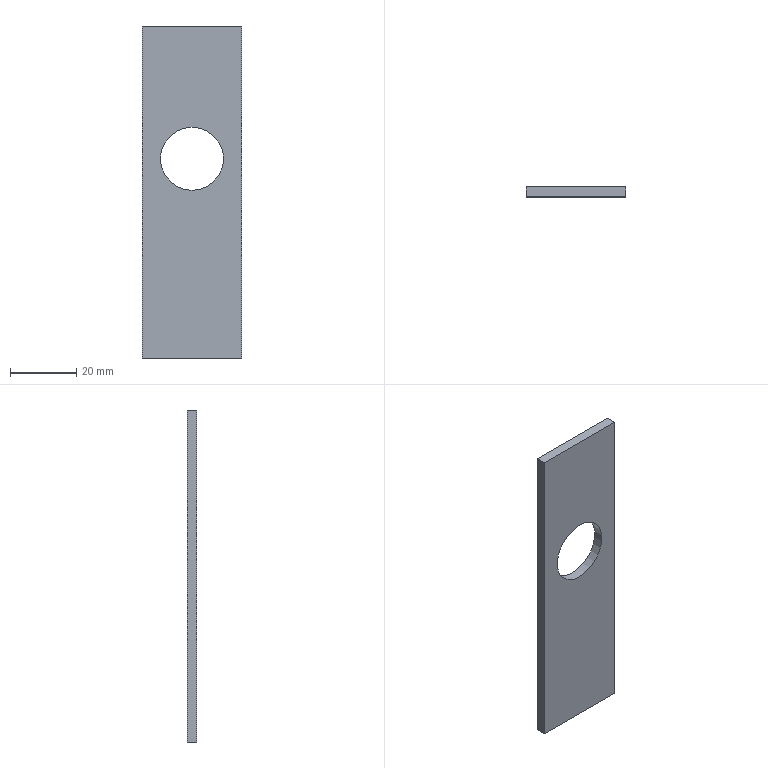Part | STEP file | 7471205 | 1 solid | 7 faces | box 30 x 3 x 100 mm | volume 8149 mm3 | plane 6 | cylinder 1 | commonest cylinder face diameters 19 x1
STEP:
#1=CARTESIAN_POINT('',(0.,0.,0.));
#2=DIRECTION('',(0.,0.,1.));
#3=DIRECTION('',(1.,0.,0.));
#4=AXIS2_PLACEMENT_3D('',#1,#2,#3);
#5=CARTESIAN_POINT('',(-15.,0.,-50.));
#6=VERTEX_POINT('',#5);
#7=CARTESIAN_POINT('',(-15.,0.,50.));
#8=VERTEX_POINT('',#7);
#9=CARTESIAN_POINT('',(-15.,0.,-50.));
#10=DIRECTION('',(0.,0.,1.));
#11=VECTOR('',#10,1.);
#12=LINE('',#9,#11);
#13=CARTESIAN_POINT('',(-15.,3.,-50.));
#14=DIRECTION('',(1.,0.,0.));
#15=DIRECTION('',(0.,0.,-1.));
#16=AXIS2_PLACEMENT_3D('',#13,#14,#15);
#17=PLANE('',#16);
#18=CARTESIAN_POINT('',(0.,-3.));
#19=DIRECTION('',(-1.,0.));
#20=VECTOR('',#19,1.);
#21=LINE('',#18,#20);
#22=(GEOMETRIC_REPRESENTATION_CONTEXT(2)PARAMETRIC_REPRESENTATION_CONTEXT()REPRESENTATION_CONTEXT('',''));
#23=DEFINITIONAL_REPRESENTATION('',(#21),#22);
#24=PCURVE('',#17,#23);
#25=CARTESIAN_POINT('',(0.,0.,0.));
#26=DIRECTION('',(0.,1.,0.));
#27=DIRECTION('',(0.,0.,1.));
#28=AXIS2_PLACEMENT_3D('',#25,#26,#27);
#29=PLANE('',#28);
#30=CARTESIAN_POINT('',(-50.,-15.));
#31=DIRECTION('',(1.,0.));
#32=VECTOR('',#31,1.);
#33=LINE('',#30,#32);
#34=(GEOMETRIC_REPRESENTATION_CONTEXT(2)PARAMETRIC_REPRESENTATION_CONTEXT()REPRESENTATION_CONTEXT('',''));
#35=DEFINITIONAL_REPRESENTATION('',(#33),#34);
#36=PCURVE('',#29,#35);
#37=SURFACE_CURVE('',#12,(#24,#36),.PCURVE_S1.);
#38=EDGE_CURVE('',#6,#8,#37,.T.);
#39=ORIENTED_EDGE('',*,*,#38,.T.);
#40=CARTESIAN_POINT('',(-15.,3.,50.));
#41=VERTEX_POINT('',#40);
#42=CARTESIAN_POINT('',(-15.,3.,50.));
#43=DIRECTION('',(0.,-1.,0.));
#44=VECTOR('',#43,1.);
#45=LINE('',#42,#44);
#46=CARTESIAN_POINT('',(-100.,0.));
#47=DIRECTION('',(0.,-1.));
#48=VECTOR('',#47,1.);
#49=LINE('',#46,#48);
#50=(GEOMETRIC_REPRESENTATION_CONTEXT(2)PARAMETRIC_REPRESENTATION_CONTEXT()REPRESENTATION_CONTEXT('',''));
#51=DEFINITIONAL_REPRESENTATION('',(#49),#50);
#52=PCURVE('',#17,#51);
#53=CARTESIAN_POINT('',(-15.,3.,50.));
#54=DIRECTION('',(0.,0.,-1.));
#55=DIRECTION('',(-1.,0.,0.));
#56=AXIS2_PLACEMENT_3D('',#53,#54,#55);
#57=PLANE('',#56);
#58=CARTESIAN_POINT('',(0.,0.));
#59=DIRECTION('',(0.,-1.));
#60=VECTOR('',#59,1.);
#61=LINE('',#58,#60);
#62=(GEOMETRIC_REPRESENTATION_CONTEXT(2)PARAMETRIC_REPRESENTATION_CONTEXT()REPRESENTATION_CONTEXT('',''));
#63=DEFINITIONAL_REPRESENTATION('',(#61),#62);
#64=PCURVE('',#57,#63);
#65=SURFACE_CURVE('',#45,(#52,#64),.PCURVE_S1.);
#66=EDGE_CURVE('',#41,#8,#65,.T.);
#67=ORIENTED_EDGE('',*,*,#66,.F.);
#68=CARTESIAN_POINT('',(-15.,3.,-50.));
#69=VERTEX_POINT('',#68);
#70=CARTESIAN_POINT('',(-15.,3.,-50.));
#71=DIRECTION('',(0.,0.,1.));
#72=VECTOR('',#71,1.);
#73=LINE('',#70,#72);
#74=CARTESIAN_POINT('',(0.,0.));
#75=DIRECTION('',(-1.,0.));
#76=VECTOR('',#75,1.);
#77=LINE('',#74,#76);
#78=(GEOMETRIC_REPRESENTATION_CONTEXT(2)PARAMETRIC_REPRESENTATION_CONTEXT()REPRESENTATION_CONTEXT('',''));
#79=DEFINITIONAL_REPRESENTATION('',(#77),#78);
#80=PCURVE('',#17,#79);
#81=CARTESIAN_POINT('',(0.,3.,0.));
#82=DIRECTION('',(0.,1.,0.));
#83=DIRECTION('',(0.,0.,1.));
#84=AXIS2_PLACEMENT_3D('',#81,#82,#83);
#85=PLANE('',#84);
#86=CARTESIAN_POINT('',(-50.,-15.));
#87=DIRECTION('',(1.,0.));
#88=VECTOR('',#87,1.);
#89=LINE('',#86,#88);
#90=(GEOMETRIC_REPRESENTATION_CONTEXT(2)PARAMETRIC_REPRESENTATION_CONTEXT()REPRESENTATION_CONTEXT('',''));
#91=DEFINITIONAL_REPRESENTATION('',(#89),#90);
#92=PCURVE('',#85,#91);
#93=SURFACE_CURVE('',#73,(#80,#92),.PCURVE_S1.);
#94=EDGE_CURVE('',#69,#41,#93,.T.);
#95=ORIENTED_EDGE('',*,*,#94,.F.);
#96=CARTESIAN_POINT('',(-15.,3.,-50.));
#97=DIRECTION('',(0.,-1.,0.));
#98=VECTOR('',#97,1.);
#99=LINE('',#96,#98);
#100=CARTESIAN_POINT('',(0.,0.));
#101=DIRECTION('',(0.,-1.));
#102=VECTOR('',#101,1.);
#103=LINE('',#100,#102);
#104=(GEOMETRIC_REPRESENTATION_CONTEXT(2)PARAMETRIC_REPRESENTATION_CONTEXT()REPRESENTATION_CONTEXT('',''));
#105=DEFINITIONAL_REPRESENTATION('',(#103),#104);
#106=PCURVE('',#17,#105);
#107=CARTESIAN_POINT('',(-15.,3.,-50.));
#108=DIRECTION('',(0.,0.,1.));
#109=DIRECTION('',(1.,0.,0.));
#110=AXIS2_PLACEMENT_3D('',#107,#108,#109);
#111=PLANE('',#110);
#112=CARTESIAN_POINT('',(0.,0.));
#113=DIRECTION('',(0.,-1.));
#114=VECTOR('',#113,1.);
#115=LINE('',#112,#114);
#116=(GEOMETRIC_REPRESENTATION_CONTEXT(2)PARAMETRIC_REPRESENTATION_CONTEXT()REPRESENTATION_CONTEXT('',''));
#117=DEFINITIONAL_REPRESENTATION('',(#115),#116);
#118=PCURVE('',#111,#117);
#119=SURFACE_CURVE('',#99,(#106,#118),.PCURVE_S1.);
#120=EDGE_CURVE('',#69,#6,#119,.T.);
#121=ORIENTED_EDGE('',*,*,#120,.T.);
#122=EDGE_LOOP('',(#39,#67,#95,#121));
#123=FACE_BOUND('',#122,.T.);
#124=ADVANCED_FACE('',(#123),#17,.F.);
#125=CARTESIAN_POINT('',(15.,0.,50.));
#126=VERTEX_POINT('',#125);
#127=CARTESIAN_POINT('',(-15.,0.,50.));
#128=DIRECTION('',(1.,0.,0.));
#129=VECTOR('',#128,1.);
#130=LINE('',#127,#129);
#131=CARTESIAN_POINT('',(0.,-3.));
#132=DIRECTION('',(-1.,0.));
#133=VECTOR('',#132,1.);
#134=LINE('',#131,#133);
#135=(GEOMETRIC_REPRESENTATION_CONTEXT(2)PARAMETRIC_REPRESENTATION_CONTEXT()REPRESENTATION_CONTEXT('',''));
#136=DEFINITIONAL_REPRESENTATION('',(#134),#135);
#137=PCURVE('',#57,#136);
#138=CARTESIAN_POINT('',(50.,-15.));
#139=DIRECTION('',(0.,1.));
#140=VECTOR('',#139,1.);
#141=LINE('',#138,#140);
#142=(GEOMETRIC_REPRESENTATION_CONTEXT(2)PARAMETRIC_REPRESENTATION_CONTEXT()REPRESENTATION_CONTEXT('',''));
#143=DEFINITIONAL_REPRESENTATION('',(#141),#142);
#144=PCURVE('',#29,#143);
#145=SURFACE_CURVE('',#130,(#137,#144),.PCURVE_S1.);
#146=EDGE_CURVE('',#8,#126,#145,.T.);
#147=ORIENTED_EDGE('',*,*,#146,.T.);
#148=CARTESIAN_POINT('',(15.,3.,50.));
#149=VERTEX_POINT('',#148);
#150=CARTESIAN_POINT('',(15.,3.,50.));
#151=DIRECTION('',(0.,-1.,0.));
#152=VECTOR('',#151,1.);
#153=LINE('',#150,#152);
#154=CARTESIAN_POINT('',(-30.,0.));
#155=DIRECTION('',(0.,-1.));
#156=VECTOR('',#155,1.);
#157=LINE('',#154,#156);
#158=(GEOMETRIC_REPRESENTATION_CONTEXT(2)PARAMETRIC_REPRESENTATION_CONTEXT()REPRESENTATION_CONTEXT('',''));
#159=DEFINITIONAL_REPRESENTATION('',(#157),#158);
#160=PCURVE('',#57,#159);
#161=CARTESIAN_POINT('',(15.,3.,-50.));
#162=DIRECTION('',(-1.,0.,0.));
#163=DIRECTION('',(0.,0.,1.));
#164=AXIS2_PLACEMENT_3D('',#161,#162,#163);
#165=PLANE('',#164);
#166=CARTESIAN_POINT('',(100.,0.));
#167=DIRECTION('',(0.,-1.));
#168=VECTOR('',#167,1.);
#169=LINE('',#166,#168);
#170=(GEOMETRIC_REPRESENTATION_CONTEXT(2)PARAMETRIC_REPRESENTATION_CONTEXT()REPRESENTATION_CONTEXT('',''));
#171=DEFINITIONAL_REPRESENTATION('',(#169),#170);
#172=PCURVE('',#165,#171);
#173=SURFACE_CURVE('',#153,(#160,#172),.PCURVE_S1.);
#174=EDGE_CURVE('',#149,#126,#173,.T.);
#175=ORIENTED_EDGE('',*,*,#174,.F.);
#176=CARTESIAN_POINT('',(-15.,3.,50.));
#177=DIRECTION('',(1.,0.,0.));
#178=VECTOR('',#177,1.);
#179=LINE('',#176,#178);
#180=CARTESIAN_POINT('',(0.,0.));
#181=DIRECTION('',(-1.,0.));
#182=VECTOR('',#181,1.);
#183=LINE('',#180,#182);
#184=(GEOMETRIC_REPRESENTATION_CONTEXT(2)PARAMETRIC_REPRESENTATION_CONTEXT()REPRESENTATION_CONTEXT('',''));
#185=DEFINITIONAL_REPRESENTATION('',(#183),#184);
#186=PCURVE('',#57,#185);
#187=CARTESIAN_POINT('',(50.,-15.));
#188=DIRECTION('',(0.,1.));
#189=VECTOR('',#188,1.);
#190=LINE('',#187,#189);
#191=(GEOMETRIC_REPRESENTATION_CONTEXT(2)PARAMETRIC_REPRESENTATION_CONTEXT()REPRESENTATION_CONTEXT('',''));
#192=DEFINITIONAL_REPRESENTATION('',(#190),#191);
#193=PCURVE('',#85,#192);
#194=SURFACE_CURVE('',#179,(#186,#193),.PCURVE_S1.);
#195=EDGE_CURVE('',#41,#149,#194,.T.);
#196=ORIENTED_EDGE('',*,*,#195,.F.);
#197=ORIENTED_EDGE('',*,*,#66,.T.);
#198=EDGE_LOOP('',(#147,#175,#196,#197));
#199=FACE_BOUND('',#198,.T.);
#200=ADVANCED_FACE('',(#199),#57,.F.);
#201=CARTESIAN_POINT('',(15.,0.,-50.));
#202=VERTEX_POINT('',#201);
#203=CARTESIAN_POINT('',(15.,0.,-50.));
#204=DIRECTION('',(0.,0.,-1.));
#205=VECTOR('',#204,1.);
#206=LINE('',#203,#205);
#207=CARTESIAN_POINT('',(0.,-3.));
#208=DIRECTION('',(-1.,0.));
#209=VECTOR('',#208,1.);
#210=LINE('',#207,#209);
#211=(GEOMETRIC_REPRESENTATION_CONTEXT(2)PARAMETRIC_REPRESENTATION_CONTEXT()REPRESENTATION_CONTEXT('',''));
#212=DEFINITIONAL_REPRESENTATION('',(#210),#211);
#213=PCURVE('',#165,#212);
#214=CARTESIAN_POINT('',(-50.,15.));
#215=DIRECTION('',(-1.,0.));
#216=VECTOR('',#215,1.);
#217=LINE('',#214,#216);
#218=(GEOMETRIC_REPRESENTATION_CONTEXT(2)PARAMETRIC_REPRESENTATION_CONTEXT()REPRESENTATION_CONTEXT('',''));
#219=DEFINITIONAL_REPRESENTATION('',(#217),#218);
#220=PCURVE('',#29,#219);
#221=SURFACE_CURVE('',#206,(#213,#220),.PCURVE_S1.);
#222=EDGE_CURVE('',#126,#202,#221,.T.);
#223=ORIENTED_EDGE('',*,*,#222,.T.);
#224=CARTESIAN_POINT('',(15.,3.,-50.));
#225=VERTEX_POINT('',#224);
#226=CARTESIAN_POINT('',(15.,3.,-50.));
#227=DIRECTION('',(0.,-1.,0.));
#228=VECTOR('',#227,1.);
#229=LINE('',#226,#228);
#230=CARTESIAN_POINT('',(0.,0.));
#231=DIRECTION('',(0.,-1.));
#232=VECTOR('',#231,1.);
#233=LINE('',#230,#232);
#234=(GEOMETRIC_REPRESENTATION_CONTEXT(2)PARAMETRIC_REPRESENTATION_CONTEXT()REPRESENTATION_CONTEXT('',''));
#235=DEFINITIONAL_REPRESENTATION('',(#233),#234);
#236=PCURVE('',#165,#235);
#237=CARTESIAN_POINT('',(30.,0.));
#238=DIRECTION('',(0.,-1.));
#239=VECTOR('',#238,1.);
#240=LINE('',#237,#239);
#241=(GEOMETRIC_REPRESENTATION_CONTEXT(2)PARAMETRIC_REPRESENTATION_CONTEXT()REPRESENTATION_CONTEXT('',''));
#242=DEFINITIONAL_REPRESENTATION('',(#240),#241);
#243=PCURVE('',#111,#242);
#244=SURFACE_CURVE('',#229,(#236,#243),.PCURVE_S1.);
#245=EDGE_CURVE('',#225,#202,#244,.T.);
#246=ORIENTED_EDGE('',*,*,#245,.F.);
#247=CARTESIAN_POINT('',(15.,3.,-50.));
#248=DIRECTION('',(0.,0.,-1.));
#249=VECTOR('',#248,1.);
#250=LINE('',#247,#249);
#251=CARTESIAN_POINT('',(0.,0.));
#252=DIRECTION('',(-1.,0.));
#253=VECTOR('',#252,1.);
#254=LINE('',#251,#253);
#255=(GEOMETRIC_REPRESENTATION_CONTEXT(2)PARAMETRIC_REPRESENTATION_CONTEXT()REPRESENTATION_CONTEXT('',''));
#256=DEFINITIONAL_REPRESENTATION('',(#254),#255);
#257=PCURVE('',#165,#256);
#258=CARTESIAN_POINT('',(-50.,15.));
#259=DIRECTION('',(-1.,0.));
#260=VECTOR('',#259,1.);
#261=LINE('',#258,#260);
#262=(GEOMETRIC_REPRESENTATION_CONTEXT(2)PARAMETRIC_REPRESENTATION_CONTEXT()REPRESENTATION_CONTEXT('',''));
#263=DEFINITIONAL_REPRESENTATION('',(#261),#262);
#264=PCURVE('',#85,#263);
#265=SURFACE_CURVE('',#250,(#257,#264),.PCURVE_S1.);
#266=EDGE_CURVE('',#149,#225,#265,.T.);
#267=ORIENTED_EDGE('',*,*,#266,.F.);
#268=ORIENTED_EDGE('',*,*,#174,.T.);
#269=EDGE_LOOP('',(#223,#246,#267,#268));
#270=FACE_BOUND('',#269,.T.);
#271=ADVANCED_FACE('',(#270),#165,.F.);
#272=CARTESIAN_POINT('',(-15.,0.,-50.));
#273=DIRECTION('',(-1.,0.,0.));
#274=VECTOR('',#273,1.);
#275=LINE('',#272,#274);
#276=CARTESIAN_POINT('',(0.,-3.));
#277=DIRECTION('',(-1.,0.));
#278=VECTOR('',#277,1.);
#279=LINE('',#276,#278);
#280=(GEOMETRIC_REPRESENTATION_CONTEXT(2)PARAMETRIC_REPRESENTATION_CONTEXT()REPRESENTATION_CONTEXT('',''));
#281=DEFINITIONAL_REPRESENTATION('',(#279),#280);
#282=PCURVE('',#111,#281);
#283=CARTESIAN_POINT('',(-50.,-15.));
#284=DIRECTION('',(0.,-1.));
#285=VECTOR('',#284,1.);
#286=LINE('',#283,#285);
#287=(GEOMETRIC_REPRESENTATION_CONTEXT(2)PARAMETRIC_REPRESENTATION_CONTEXT()REPRESENTATION_CONTEXT('',''));
#288=DEFINITIONAL_REPRESENTATION('',(#286),#287);
#289=PCURVE('',#29,#288);
#290=SURFACE_CURVE('',#275,(#282,#289),.PCURVE_S1.);
#291=EDGE_CURVE('',#202,#6,#290,.T.);
#292=ORIENTED_EDGE('',*,*,#291,.T.);
#293=ORIENTED_EDGE('',*,*,#120,.F.);
#294=CARTESIAN_POINT('',(-15.,3.,-50.));
#295=DIRECTION('',(-1.,0.,0.));
#296=VECTOR('',#295,1.);
#297=LINE('',#294,#296);
#298=CARTESIAN_POINT('',(0.,0.));
#299=DIRECTION('',(-1.,0.));
#300=VECTOR('',#299,1.);
#301=LINE('',#298,#300);
#302=(GEOMETRIC_REPRESENTATION_CONTEXT(2)PARAMETRIC_REPRESENTATION_CONTEXT()REPRESENTATION_CONTEXT('',''));
#303=DEFINITIONAL_REPRESENTATION('',(#301),#302);
#304=PCURVE('',#111,#303);
#305=CARTESIAN_POINT('',(-50.,-15.));
#306=DIRECTION('',(0.,-1.));
#307=VECTOR('',#306,1.);
#308=LINE('',#305,#307);
#309=(GEOMETRIC_REPRESENTATION_CONTEXT(2)PARAMETRIC_REPRESENTATION_CONTEXT()REPRESENTATION_CONTEXT('',''));
#310=DEFINITIONAL_REPRESENTATION('',(#308),#309);
#311=PCURVE('',#85,#310);
#312=SURFACE_CURVE('',#297,(#304,#311),.PCURVE_S1.);
#313=EDGE_CURVE('',#225,#69,#312,.T.);
#314=ORIENTED_EDGE('',*,*,#313,.F.);
#315=ORIENTED_EDGE('',*,*,#245,.T.);
#316=EDGE_LOOP('',(#292,#293,#314,#315));
#317=FACE_BOUND('',#316,.T.);
#318=ADVANCED_FACE('',(#317),#111,.F.);
#319=CARTESIAN_POINT('',(0.,3.,19.5));
#320=VERTEX_POINT('',#319);
#321=CARTESIAN_POINT('',(0.,3.,10.));
#322=DIRECTION('',(0.,1.,0.));
#323=DIRECTION('',(0.,0.,1.));
#324=AXIS2_PLACEMENT_3D('',#321,#322,#323);
#325=CIRCLE('',#324,9.5);
#326=CARTESIAN_POINT('',(10.,0.));
#327=DIRECTION('',(1.,0.));
#328=AXIS2_PLACEMENT_2D('',#326,#327);
#329=CIRCLE('',#328,9.5);
#330=(GEOMETRIC_REPRESENTATION_CONTEXT(2)PARAMETRIC_REPRESENTATION_CONTEXT()REPRESENTATION_CONTEXT('',''));
#331=DEFINITIONAL_REPRESENTATION('',(#329),#330);
#332=PCURVE('',#85,#331);
#333=CARTESIAN_POINT('',(0.,-7.,10.));
#334=DIRECTION('',(0.,1.,0.));
#335=DIRECTION('',(0.,0.,1.));
#336=AXIS2_PLACEMENT_3D('',#333,#334,#335);
#337=CYLINDRICAL_SURFACE('',#336,9.5);
#338=CARTESIAN_POINT('',(0.,10.));
#339=DIRECTION('',(1.,0.));
#340=VECTOR('',#339,1.);
#341=LINE('',#338,#340);
#342=(GEOMETRIC_REPRESENTATION_CONTEXT(2)PARAMETRIC_REPRESENTATION_CONTEXT()REPRESENTATION_CONTEXT('',''));
#343=DEFINITIONAL_REPRESENTATION('',(#341),#342);
#344=PCURVE('',#337,#343);
#345=SURFACE_CURVE('',#325,(#332,#344),.PCURVE_S1.);
#346=EDGE_CURVE('',#320,#320,#345,.T.);
#347=ORIENTED_EDGE('',*,*,#346,.F.);
#348=EDGE_LOOP('',(#347));
#349=FACE_BOUND('',#348,.T.);
#350=ORIENTED_EDGE('',*,*,#94,.T.);
#351=ORIENTED_EDGE('',*,*,#195,.T.);
#352=ORIENTED_EDGE('',*,*,#266,.T.);
#353=ORIENTED_EDGE('',*,*,#313,.T.);
#354=EDGE_LOOP('',(#350,#351,#352,#353));
#355=FACE_BOUND('',#354,.T.);
#356=ADVANCED_FACE('',(#349,#355),#85,.T.);
#357=CARTESIAN_POINT('',(0.,0.,19.5));
#358=VERTEX_POINT('',#357);
#359=CARTESIAN_POINT('',(0.,0.,10.));
#360=DIRECTION('',(0.,1.,0.));
#361=DIRECTION('',(0.,0.,1.));
#362=AXIS2_PLACEMENT_3D('',#359,#360,#361);
#363=CIRCLE('',#362,9.5);
#364=CARTESIAN_POINT('',(10.,0.));
#365=DIRECTION('',(1.,0.));
#366=AXIS2_PLACEMENT_2D('',#364,#365);
#367=CIRCLE('',#366,9.5);
#368=(GEOMETRIC_REPRESENTATION_CONTEXT(2)PARAMETRIC_REPRESENTATION_CONTEXT()REPRESENTATION_CONTEXT('',''));
#369=DEFINITIONAL_REPRESENTATION('',(#367),#368);
#370=PCURVE('',#29,#369);
#371=CARTESIAN_POINT('',(0.,7.));
#372=DIRECTION('',(1.,0.));
#373=VECTOR('',#372,1.);
#374=LINE('',#371,#373);
#375=(GEOMETRIC_REPRESENTATION_CONTEXT(2)PARAMETRIC_REPRESENTATION_CONTEXT()REPRESENTATION_CONTEXT('',''));
#376=DEFINITIONAL_REPRESENTATION('',(#374),#375);
#377=PCURVE('',#337,#376);
#378=SURFACE_CURVE('',#363,(#370,#377),.PCURVE_S1.);
#379=EDGE_CURVE('',#358,#358,#378,.T.);
#380=ORIENTED_EDGE('',*,*,#379,.T.);
#381=EDGE_LOOP('',(#380));
#382=FACE_BOUND('',#381,.T.);
#383=ORIENTED_EDGE('',*,*,#38,.F.);
#384=ORIENTED_EDGE('',*,*,#291,.F.);
#385=ORIENTED_EDGE('',*,*,#222,.F.);
#386=ORIENTED_EDGE('',*,*,#146,.F.);
#387=EDGE_LOOP('',(#383,#384,#385,#386));
#388=FACE_BOUND('',#387,.T.);
#389=ADVANCED_FACE('',(#382,#388),#29,.F.);
#390=ORIENTED_EDGE('',*,*,#346,.F.);
#391=CARTESIAN_POINT('',(0.,0.,19.5));
#392=CARTESIAN_POINT('',(0.,3.,19.5));
#393=B_SPLINE_CURVE_WITH_KNOTS('',1,(#391,#392),.UNSPECIFIED.,.F.,.F.,(2,2),(7.,10.),.PIECEWISE_BEZIER_KNOTS.);
#394=CARTESIAN_POINT('',(0.,0.));
#395=DIRECTION('',(0.,1.));
#396=VECTOR('',#395,1.);
#397=LINE('',#394,#396);
#398=(GEOMETRIC_REPRESENTATION_CONTEXT(2)PARAMETRIC_REPRESENTATION_CONTEXT()REPRESENTATION_CONTEXT('',''));
#399=DEFINITIONAL_REPRESENTATION('',(#397),#398);
#400=PCURVE('',#337,#399);
#401=CARTESIAN_POINT('',(6.283,0.));
#402=DIRECTION('',(0.,1.));
#403=VECTOR('',#402,1.);
#404=LINE('',#401,#403);
#405=(GEOMETRIC_REPRESENTATION_CONTEXT(2)PARAMETRIC_REPRESENTATION_CONTEXT()REPRESENTATION_CONTEXT('',''));
#406=DEFINITIONAL_REPRESENTATION('',(#404),#405);
#407=PCURVE('',#337,#406);
#408=SEAM_CURVE('',#393,(#400,#407),.PCURVE_S1.);
#409=EDGE_CURVE('',#358,#320,#408,.T.);
#410=ORIENTED_EDGE('',*,*,#409,.F.);
#411=ORIENTED_EDGE('',*,*,#379,.T.);
#412=ORIENTED_EDGE('',*,*,#409,.T.);
#413=EDGE_LOOP('',(#390,#410,#411,#412));
#414=FACE_BOUND('',#413,.F.);
#415=ADVANCED_FACE('',(#414),#337,.F.);
#416=CLOSED_SHELL('',(#124,#200,#271,#318,#356,#389,#415));
#417=MANIFOLD_SOLID_BREP('',#416);
#418=(LENGTH_UNIT()NAMED_UNIT(*)SI_UNIT(.MILLI.,.METRE.));
#419=UNCERTAINTY_MEASURE_WITH_UNIT(LENGTH_MEASURE(0.000002),#418,'','');
#420=(NAMED_UNIT(*)PLANE_ANGLE_UNIT()SI_UNIT($,.RADIAN.));
#421=(NAMED_UNIT(*)SI_UNIT($,.STERADIAN.)SOLID_ANGLE_UNIT());
#422=(GEOMETRIC_REPRESENTATION_CONTEXT(3)GLOBAL_UNCERTAINTY_ASSIGNED_CONTEXT((#419))GLOBAL_UNIT_ASSIGNED_CONTEXT((#418,#420,#421))REPRESENTATION_CONTEXT('',''));
#423=ADVANCED_BREP_SHAPE_REPRESENTATION('',(#4,#417),#422);